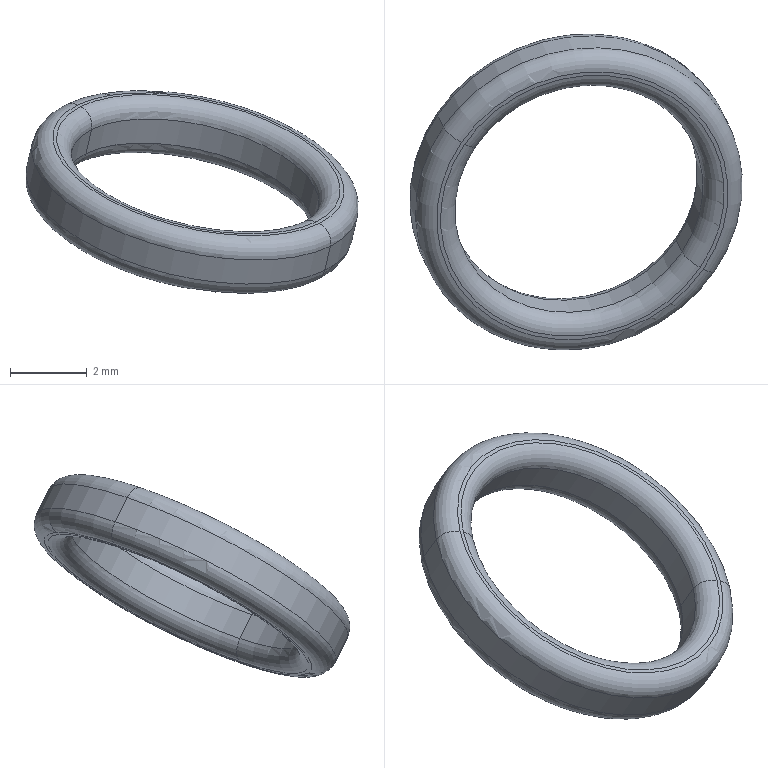Part | SolidWorks | features BaseBody 1 | 1 solid | 14 faces | box 8.65 x 8.202 x 5.272 mm | volume 36.271 mm3 | torus 8 | cylinder 4 | plane 2 | commonest cylinder face diameters 6.6 x2 8.665 x2
STEP:
#1=CARTESIAN_POINT('',(1964.802,-244.96,1000.506));
#2=VERTEX_POINT('',#1);
#3=CARTESIAN_POINT('',(1970.925,-248.162,997.508));
#4=VERTEX_POINT('',#3);
#5=CARTESIAN_POINT('',(1967.864,-246.561,999.007));
#6=DIRECTION('',(-0.2015,0.436,-0.8771));
#7=DIRECTION('',(-0.9754,-0.007201,0.2205));
#8=AXIS2_PLACEMENT_3D('',#5,#6,#7);
#9=CIRCLE('',#8,3.766);
#10=EDGE_CURVE('',#2,#4,#9,.T.);
#11=ORIENTED_EDGE('',*,*,#10,.F.);
#12=CARTESIAN_POINT('',(1965.087,-244.955,999.912));
#13=VERTEX_POINT('',#12);
#14=CARTESIAN_POINT('',(1964.708,-244.757,1000.097));
#15=DIRECTION('',(-0.5464,-0.7932,-0.2688));
#16=DIRECTION('',(-0.8129,0.4251,0.3981));
#17=AXIS2_PLACEMENT_3D('',#14,#15,#16);
#18=CIRCLE('',#17,0.4662);
#19=EDGE_CURVE('',#13,#2,#18,.T.);
#20=ORIENTED_EDGE('',*,*,#19,.F.);
#21=CARTESIAN_POINT('',(1970.452,-247.761,997.284));
#22=VERTEX_POINT('',#21);
#23=CARTESIAN_POINT('',(1967.77,-246.358,998.598));
#24=DIRECTION('',(-0.2015,0.436,-0.8771));
#25=DIRECTION('',(-0.9754,-0.007201,0.2205));
#26=AXIS2_PLACEMENT_3D('',#23,#24,#25);
#27=CIRCLE('',#26,3.3);
#28=EDGE_CURVE('',#13,#22,#27,.T.);
#29=ORIENTED_EDGE('',*,*,#28,.T.);
#30=CARTESIAN_POINT('',(1970.831,-247.959,997.099));
#31=DIRECTION('',(-0.5464,-0.7932,-0.2688));
#32=DIRECTION('',(-0.8129,0.4251,0.3981));
#33=AXIS2_PLACEMENT_3D('',#30,#31,#32);
#34=CIRCLE('',#33,0.4663);
#35=EDGE_CURVE('',#4,#22,#34,.T.);
#36=ORIENTED_EDGE('',*,*,#35,.F.);
#37=EDGE_LOOP('',(#11,#20,#29,#36));
#38=FACE_OUTER_BOUND('',#37,.T.);
#39=CARTESIAN_POINT('',(1967.77,-246.358,998.598));
#40=DIRECTION('',(-0.2015,0.436,-0.8771));
#41=DIRECTION('',(0.8129,-0.4251,-0.3981));
#42=AXIS2_PLACEMENT_3D('',#39,#40,#41);
#43=TOROIDAL_SURFACE('',#42,3.766,0.4662);
#44=ADVANCED_FACE('',(#38),#43,.T.);
#45=CARTESIAN_POINT('',(1967.864,-246.561,999.007));
#46=DIRECTION('',(-0.2015,0.436,-0.8771));
#47=DIRECTION('',(-0.9754,-0.007201,0.2205));
#48=AXIS2_PLACEMENT_3D('',#45,#46,#47);
#49=CIRCLE('',#48,3.766);
#50=EDGE_CURVE('',#4,#2,#49,.T.);
#51=ORIENTED_EDGE('',*,*,#50,.F.);
#52=ORIENTED_EDGE('',*,*,#35,.T.);
#53=CARTESIAN_POINT('',(1967.77,-246.358,998.598));
#54=DIRECTION('',(-0.2015,0.436,-0.8771));
#55=DIRECTION('',(-0.9754,-0.007201,0.2205));
#56=AXIS2_PLACEMENT_3D('',#53,#54,#55);
#57=CIRCLE('',#56,3.3);
#58=EDGE_CURVE('',#22,#13,#57,.T.);
#59=ORIENTED_EDGE('',*,*,#58,.T.);
#60=ORIENTED_EDGE('',*,*,#19,.T.);
#61=EDGE_LOOP('',(#51,#52,#59,#60));
#62=FACE_OUTER_BOUND('',#61,.T.);
#63=CARTESIAN_POINT('',(1967.77,-246.358,998.598));
#64=DIRECTION('',(-0.2015,0.436,-0.8771));
#65=DIRECTION('',(0.8129,-0.4251,-0.3981));
#66=AXIS2_PLACEMENT_3D('',#63,#64,#65);
#67=TOROIDAL_SURFACE('',#66,3.766,0.4662);
#68=ADVANCED_FACE('',(#62),#67,.T.);
#69=ORIENTED_EDGE('',*,*,#28,.F.);
#70=CARTESIAN_POINT('',(1964.943,-244.644,999.286));
#71=VERTEX_POINT('',#70);
#72=CARTESIAN_POINT('',(1965.015,-244.8,999.599));
#73=DIRECTION('',(-0.2015,0.436,-0.8771));
#74=VECTOR('',#73,1000.);
#75=LINE('',#72,#74);
#76=EDGE_CURVE('',#13,#71,#75,.T.);
#77=ORIENTED_EDGE('',*,*,#76,.T.);
#78=CARTESIAN_POINT('',(1970.309,-247.45,996.659));
#79=VERTEX_POINT('',#78);
#80=CARTESIAN_POINT('',(1967.626,-246.047,997.973));
#81=DIRECTION('',(-0.2015,0.436,-0.8771));
#82=DIRECTION('',(-0.9754,-0.007201,0.2205));
#83=AXIS2_PLACEMENT_3D('',#80,#81,#82);
#84=CIRCLE('',#83,3.3);
#85=EDGE_CURVE('',#71,#79,#84,.T.);
#86=ORIENTED_EDGE('',*,*,#85,.T.);
#87=CARTESIAN_POINT('',(1970.38,-247.605,996.972));
#88=DIRECTION('',(0.2015,-0.436,0.8771));
#89=VECTOR('',#88,1000.);
#90=LINE('',#87,#89);
#91=EDGE_CURVE('',#79,#22,#90,.T.);
#92=ORIENTED_EDGE('',*,*,#91,.T.);
#93=EDGE_LOOP('',(#69,#77,#86,#92));
#94=FACE_OUTER_BOUND('',#93,.T.);
#95=CARTESIAN_POINT('',(1967.698,-246.203,998.285));
#96=DIRECTION('',(-0.2015,0.436,-0.8771));
#97=DIRECTION('',(0.8129,-0.4251,-0.3981));
#98=AXIS2_PLACEMENT_3D('',#95,#96,#97);
#99=CYLINDRICAL_SURFACE('',#98,3.3);
#100=ADVANCED_FACE('',(#94),#99,.F.);
#101=ORIENTED_EDGE('',*,*,#58,.F.);
#102=ORIENTED_EDGE('',*,*,#91,.F.);
#103=CARTESIAN_POINT('',(1967.626,-246.047,997.973));
#104=DIRECTION('',(-0.2015,0.436,-0.8771));
#105=DIRECTION('',(-0.9754,-0.007201,0.2205));
#106=AXIS2_PLACEMENT_3D('',#103,#104,#105);
#107=CIRCLE('',#106,3.3);
#108=EDGE_CURVE('',#79,#71,#107,.T.);
#109=ORIENTED_EDGE('',*,*,#108,.T.);
#110=ORIENTED_EDGE('',*,*,#76,.F.);
#111=EDGE_LOOP('',(#101,#102,#109,#110));
#112=FACE_OUTER_BOUND('',#111,.T.);
#113=CARTESIAN_POINT('',(1967.698,-246.203,998.285));
#114=DIRECTION('',(-0.2015,0.436,-0.8771));
#115=DIRECTION('',(0.8129,-0.4251,-0.3981));
#116=AXIS2_PLACEMENT_3D('',#113,#114,#115);
#117=CYLINDRICAL_SURFACE('',#116,3.3);
#118=ADVANCED_FACE('',(#112),#117,.F.);
#119=ORIENTED_EDGE('',*,*,#85,.F.);
#120=CARTESIAN_POINT('',(1964.47,-244.243,999.063));
#121=VERTEX_POINT('',#120);
#122=CARTESIAN_POINT('',(1964.564,-244.446,999.472));
#123=DIRECTION('',(-0.5464,-0.7932,-0.2688));
#124=DIRECTION('',(-0.8129,0.4251,0.3981));
#125=AXIS2_PLACEMENT_3D('',#122,#123,#124);
#126=CIRCLE('',#125,0.4663);
#127=EDGE_CURVE('',#121,#71,#126,.T.);
#128=ORIENTED_EDGE('',*,*,#127,.F.);
#129=CARTESIAN_POINT('',(1970.594,-247.445,996.064));
#130=VERTEX_POINT('',#129);
#131=CARTESIAN_POINT('',(1967.532,-245.844,997.564));
#132=DIRECTION('',(-0.2015,0.436,-0.8771));
#133=DIRECTION('',(-0.9754,-0.007201,0.2205));
#134=AXIS2_PLACEMENT_3D('',#131,#132,#133);
#135=CIRCLE('',#134,3.766);
#136=EDGE_CURVE('',#121,#130,#135,.T.);
#137=ORIENTED_EDGE('',*,*,#136,.T.);
#138=CARTESIAN_POINT('',(1970.688,-247.648,996.473));
#139=DIRECTION('',(-0.5464,-0.7932,-0.2688));
#140=DIRECTION('',(-0.8129,0.4251,0.3981));
#141=AXIS2_PLACEMENT_3D('',#138,#139,#140);
#142=CIRCLE('',#141,0.4663);
#143=EDGE_CURVE('',#79,#130,#142,.T.);
#144=ORIENTED_EDGE('',*,*,#143,.F.);
#145=EDGE_LOOP('',(#119,#128,#137,#144));
#146=FACE_OUTER_BOUND('',#145,.T.);
#147=CARTESIAN_POINT('',(1967.626,-246.047,997.973));
#148=DIRECTION('',(-0.2015,0.436,-0.8771));
#149=DIRECTION('',(0.8129,-0.4251,-0.3981));
#150=AXIS2_PLACEMENT_3D('',#147,#148,#149);
#151=TOROIDAL_SURFACE('',#150,3.766,0.4662);
#152=ADVANCED_FACE('',(#146),#151,.T.);
#153=ORIENTED_EDGE('',*,*,#108,.F.);
#154=ORIENTED_EDGE('',*,*,#143,.T.);
#155=CARTESIAN_POINT('',(1967.532,-245.844,997.564));
#156=DIRECTION('',(-0.2015,0.436,-0.8771));
#157=DIRECTION('',(-0.9754,-0.007201,0.2205));
#158=AXIS2_PLACEMENT_3D('',#155,#156,#157);
#159=CIRCLE('',#158,3.766);
#160=EDGE_CURVE('',#130,#121,#159,.T.);
#161=ORIENTED_EDGE('',*,*,#160,.T.);
#162=ORIENTED_EDGE('',*,*,#127,.T.);
#163=EDGE_LOOP('',(#153,#154,#161,#162));
#164=FACE_OUTER_BOUND('',#163,.T.);
#165=CARTESIAN_POINT('',(1967.626,-246.047,997.973));
#166=DIRECTION('',(-0.2015,0.436,-0.8771));
#167=DIRECTION('',(0.8129,-0.4251,-0.3981));
#168=AXIS2_PLACEMENT_3D('',#165,#166,#167);
#169=TOROIDAL_SURFACE('',#168,3.766,0.4662);
#170=ADVANCED_FACE('',(#164),#169,.T.);
#171=CARTESIAN_POINT('',(1964.389,-244.2,999.103));
#172=VERTEX_POINT('',#171);
#173=CARTESIAN_POINT('',(1970.675,-247.487,996.025));
#174=VERTEX_POINT('',#173);
#175=CARTESIAN_POINT('',(1967.532,-245.844,997.564));
#176=DIRECTION('',(-0.2015,0.436,-0.8771));
#177=DIRECTION('',(-0.9754,-0.007201,0.2205));
#178=AXIS2_PLACEMENT_3D('',#175,#176,#177);
#179=CIRCLE('',#178,3.866);
#180=EDGE_CURVE('',#172,#174,#179,.T.);
#181=ORIENTED_EDGE('',*,*,#180,.F.);
#182=CARTESIAN_POINT('',(1964.104,-244.205,999.697));
#183=VERTEX_POINT('',#182);
#184=CARTESIAN_POINT('',(1964.483,-244.403,999.512));
#185=DIRECTION('',(-0.5464,-0.7932,-0.2688));
#186=DIRECTION('',(-0.8129,0.4251,0.3981));
#187=AXIS2_PLACEMENT_3D('',#184,#185,#186);
#188=CIRCLE('',#187,0.4662);
#189=EDGE_CURVE('',#183,#172,#188,.T.);
#190=ORIENTED_EDGE('',*,*,#189,.F.);
#191=CARTESIAN_POINT('',(1971.148,-247.889,996.248));
#192=VERTEX_POINT('',#191);
#193=CARTESIAN_POINT('',(1967.626,-246.047,997.973));
#194=DIRECTION('',(-0.2015,0.436,-0.8771));
#195=DIRECTION('',(-0.9754,-0.007201,0.2205));
#196=AXIS2_PLACEMENT_3D('',#193,#194,#195);
#197=CIRCLE('',#196,4.333);
#198=EDGE_CURVE('',#183,#192,#197,.T.);
#199=ORIENTED_EDGE('',*,*,#198,.T.);
#200=CARTESIAN_POINT('',(1970.769,-247.691,996.433));
#201=DIRECTION('',(-0.5464,-0.7932,-0.2688));
#202=DIRECTION('',(-0.8129,0.4251,0.3981));
#203=AXIS2_PLACEMENT_3D('',#200,#201,#202);
#204=CIRCLE('',#203,0.4663);
#205=EDGE_CURVE('',#174,#192,#204,.T.);
#206=ORIENTED_EDGE('',*,*,#205,.F.);
#207=EDGE_LOOP('',(#181,#190,#199,#206));
#208=FACE_OUTER_BOUND('',#207,.T.);
#209=CARTESIAN_POINT('',(1967.626,-246.047,997.973));
#210=DIRECTION('',(-0.2015,0.436,-0.8771));
#211=DIRECTION('',(0.8129,-0.4251,-0.3981));
#212=AXIS2_PLACEMENT_3D('',#209,#210,#211);
#213=TOROIDAL_SURFACE('',#212,3.866,0.4662);
#214=ADVANCED_FACE('',(#208),#213,.T.);
#215=CARTESIAN_POINT('',(1967.532,-245.844,997.564));
#216=DIRECTION('',(-0.2015,0.436,-0.8771));
#217=DIRECTION('',(-0.9754,-0.007201,0.2205));
#218=AXIS2_PLACEMENT_3D('',#215,#216,#217);
#219=CIRCLE('',#218,3.866);
#220=EDGE_CURVE('',#174,#172,#219,.T.);
#221=ORIENTED_EDGE('',*,*,#220,.F.);
#222=ORIENTED_EDGE('',*,*,#205,.T.);
#223=CARTESIAN_POINT('',(1967.626,-246.047,997.973));
#224=DIRECTION('',(-0.2015,0.436,-0.8771));
#225=DIRECTION('',(-0.9754,-0.007201,0.2205));
#226=AXIS2_PLACEMENT_3D('',#223,#224,#225);
#227=CIRCLE('',#226,4.333);
#228=EDGE_CURVE('',#192,#183,#227,.T.);
#229=ORIENTED_EDGE('',*,*,#228,.T.);
#230=ORIENTED_EDGE('',*,*,#189,.T.);
#231=EDGE_LOOP('',(#221,#222,#229,#230));
#232=FACE_OUTER_BOUND('',#231,.T.);
#233=CARTESIAN_POINT('',(1967.626,-246.047,997.973));
#234=DIRECTION('',(-0.2015,0.436,-0.8771));
#235=DIRECTION('',(0.8129,-0.4251,-0.3981));
#236=AXIS2_PLACEMENT_3D('',#233,#234,#235);
#237=TOROIDAL_SURFACE('',#236,3.866,0.4662);
#238=ADVANCED_FACE('',(#232),#237,.T.);
#239=ORIENTED_EDGE('',*,*,#198,.F.);
#240=CARTESIAN_POINT('',(1964.248,-244.516,1000.323));
#241=VERTEX_POINT('',#240);
#242=CARTESIAN_POINT('',(1964.176,-244.361,1000.01));
#243=DIRECTION('',(0.2015,-0.436,0.8771));
#244=VECTOR('',#243,1000.);
#245=LINE('',#242,#244);
#246=EDGE_CURVE('',#183,#241,#245,.T.);
#247=ORIENTED_EDGE('',*,*,#246,.T.);
#248=CARTESIAN_POINT('',(1971.292,-248.2,996.873));
#249=VERTEX_POINT('',#248);
#250=CARTESIAN_POINT('',(1967.77,-246.358,998.598));
#251=DIRECTION('',(-0.2015,0.436,-0.8771));
#252=DIRECTION('',(-0.9754,-0.007201,0.2205));
#253=AXIS2_PLACEMENT_3D('',#250,#251,#252);
#254=CIRCLE('',#253,4.333);
#255=EDGE_CURVE('',#241,#249,#254,.T.);
#256=ORIENTED_EDGE('',*,*,#255,.T.);
#257=CARTESIAN_POINT('',(1971.22,-248.044,996.561));
#258=DIRECTION('',(-0.2015,0.436,-0.8771));
#259=VECTOR('',#258,1000.);
#260=LINE('',#257,#259);
#261=EDGE_CURVE('',#249,#192,#260,.T.);
#262=ORIENTED_EDGE('',*,*,#261,.T.);
#263=EDGE_LOOP('',(#239,#247,#256,#262));
#264=FACE_OUTER_BOUND('',#263,.T.);
#265=CARTESIAN_POINT('',(1967.698,-246.203,998.285));
#266=DIRECTION('',(-0.2015,0.436,-0.8771));
#267=DIRECTION('',(0.8129,-0.4251,-0.3981));
#268=AXIS2_PLACEMENT_3D('',#265,#266,#267);
#269=CYLINDRICAL_SURFACE('',#268,4.333);
#270=ADVANCED_FACE('',(#264),#269,.T.);
#271=ORIENTED_EDGE('',*,*,#228,.F.);
#272=ORIENTED_EDGE('',*,*,#261,.F.);
#273=CARTESIAN_POINT('',(1967.77,-246.358,998.598));
#274=DIRECTION('',(-0.2015,0.436,-0.8771));
#275=DIRECTION('',(-0.9754,-0.007201,0.2205));
#276=AXIS2_PLACEMENT_3D('',#273,#274,#275);
#277=CIRCLE('',#276,4.333);
#278=EDGE_CURVE('',#249,#241,#277,.T.);
#279=ORIENTED_EDGE('',*,*,#278,.T.);
#280=ORIENTED_EDGE('',*,*,#246,.F.);
#281=EDGE_LOOP('',(#271,#272,#279,#280));
#282=FACE_OUTER_BOUND('',#281,.T.);
#283=CARTESIAN_POINT('',(1967.698,-246.203,998.285));
#284=DIRECTION('',(-0.2015,0.436,-0.8771));
#285=DIRECTION('',(0.8129,-0.4251,-0.3981));
#286=AXIS2_PLACEMENT_3D('',#283,#284,#285);
#287=CYLINDRICAL_SURFACE('',#286,4.333);
#288=ADVANCED_FACE('',(#282),#287,.T.);
#289=ORIENTED_EDGE('',*,*,#255,.F.);
#290=CARTESIAN_POINT('',(1964.721,-244.918,1000.546));
#291=VERTEX_POINT('',#290);
#292=CARTESIAN_POINT('',(1964.627,-244.714,1000.137));
#293=DIRECTION('',(0.5464,0.7932,0.2688));
#294=DIRECTION('',(-0.8129,0.4251,0.3981));
#295=AXIS2_PLACEMENT_3D('',#292,#293,#294);
#296=CIRCLE('',#295,0.4663);
#297=EDGE_CURVE('',#241,#291,#296,.T.);
#298=ORIENTED_EDGE('',*,*,#297,.T.);
#299=CARTESIAN_POINT('',(1971.006,-248.205,997.468));
#300=VERTEX_POINT('',#299);
#301=CARTESIAN_POINT('',(1967.864,-246.561,999.007));
#302=DIRECTION('',(-0.2015,0.436,-0.8771));
#303=DIRECTION('',(-0.9754,-0.007201,0.2205));
#304=AXIS2_PLACEMENT_3D('',#301,#302,#303);
#305=CIRCLE('',#304,3.866);
#306=EDGE_CURVE('',#291,#300,#305,.T.);
#307=ORIENTED_EDGE('',*,*,#306,.T.);
#308=CARTESIAN_POINT('',(1970.913,-248.002,997.059));
#309=DIRECTION('',(0.5464,0.7932,0.2688));
#310=DIRECTION('',(-0.8129,0.4251,0.3981));
#311=AXIS2_PLACEMENT_3D('',#308,#309,#310);
#312=CIRCLE('',#311,0.4662);
#313=EDGE_CURVE('',#300,#249,#312,.T.);
#314=ORIENTED_EDGE('',*,*,#313,.T.);
#315=EDGE_LOOP('',(#289,#298,#307,#314));
#316=FACE_OUTER_BOUND('',#315,.T.);
#317=CARTESIAN_POINT('',(1967.77,-246.358,998.598));
#318=DIRECTION('',(-0.2015,0.436,-0.8771));
#319=DIRECTION('',(0.8129,-0.4251,-0.3981));
#320=AXIS2_PLACEMENT_3D('',#317,#318,#319);
#321=TOROIDAL_SURFACE('',#320,3.866,0.4662);
#322=ADVANCED_FACE('',(#316),#321,.T.);
#323=ORIENTED_EDGE('',*,*,#278,.F.);
#324=ORIENTED_EDGE('',*,*,#313,.F.);
#325=CARTESIAN_POINT('',(1967.864,-246.561,999.007));
#326=DIRECTION('',(-0.2015,0.436,-0.8771));
#327=DIRECTION('',(-0.9754,-0.007201,0.2205));
#328=AXIS2_PLACEMENT_3D('',#325,#326,#327);
#329=CIRCLE('',#328,3.866);
#330=EDGE_CURVE('',#300,#291,#329,.T.);
#331=ORIENTED_EDGE('',*,*,#330,.T.);
#332=ORIENTED_EDGE('',*,*,#297,.F.);
#333=EDGE_LOOP('',(#323,#324,#331,#332));
#334=FACE_OUTER_BOUND('',#333,.T.);
#335=CARTESIAN_POINT('',(1967.77,-246.358,998.598));
#336=DIRECTION('',(-0.2015,0.436,-0.8771));
#337=DIRECTION('',(0.8129,-0.4251,-0.3981));
#338=AXIS2_PLACEMENT_3D('',#335,#336,#337);
#339=TOROIDAL_SURFACE('',#338,3.866,0.4662);
#340=ADVANCED_FACE('',(#334),#339,.T.);
#341=ORIENTED_EDGE('',*,*,#220,.T.);
#342=ORIENTED_EDGE('',*,*,#180,.T.);
#343=EDGE_LOOP('',(#341,#342));
#344=FACE_OUTER_BOUND('',#343,.T.);
#345=ORIENTED_EDGE('',*,*,#136,.F.);
#346=ORIENTED_EDGE('',*,*,#160,.F.);
#347=EDGE_LOOP('',(#345,#346));
#348=FACE_BOUND('',#347,.T.);
#349=CARTESIAN_POINT('',(1963.761,-245.872,998.416));
#350=DIRECTION('',(-0.2015,0.436,-0.8771));
#351=DIRECTION('',(0.9754,0.007201,-0.2205));
#352=AXIS2_PLACEMENT_3D('',#349,#350,#351);
#353=PLANE('',#352);
#354=ADVANCED_FACE('',(#344,#348),#353,.T.);
#355=ORIENTED_EDGE('',*,*,#306,.F.);
#356=ORIENTED_EDGE('',*,*,#330,.F.);
#357=EDGE_LOOP('',(#355,#356));
#358=FACE_OUTER_BOUND('',#357,.T.);
#359=ORIENTED_EDGE('',*,*,#50,.T.);
#360=ORIENTED_EDGE('',*,*,#10,.T.);
#361=EDGE_LOOP('',(#359,#360));
#362=FACE_BOUND('',#361,.T.);
#363=CARTESIAN_POINT('',(1964.19,-246.588,999.837));
#364=DIRECTION('',(-0.2015,0.436,-0.8771));
#365=DIRECTION('',(0.9754,0.007201,-0.2205));
#366=AXIS2_PLACEMENT_3D('',#363,#364,#365);
#367=PLANE('',#366);
#368=ADVANCED_FACE('',(#358,#362),#367,.F.);
#369=CLOSED_SHELL('',(#44,#68,#100,#118,#152,#170,#214,#238,#270,#288,#322,#340,#354,#368));
#370=MANIFOLD_SOLID_BREP('',#369);
#371=CARTESIAN_POINT('',(0.,0.,0.));
#372=DIRECTION('',(0.,0.,1.));
#373=DIRECTION('',(1.,0.,0.));
#374=AXIS2_PLACEMENT_3D('',#371,#372,#373);
#375=(LENGTH_UNIT()NAMED_UNIT(*)SI_UNIT(.MILLI.,.METRE.));
#376=UNCERTAINTY_MEASURE_WITH_UNIT(LENGTH_MEASURE(0.00001),#375,'','');
#377=(NAMED_UNIT(*)PLANE_ANGLE_UNIT()SI_UNIT($,.RADIAN.));
#378=(NAMED_UNIT(*)SI_UNIT($,.STERADIAN.)SOLID_ANGLE_UNIT());
#379=(GEOMETRIC_REPRESENTATION_CONTEXT(3)GLOBAL_UNCERTAINTY_ASSIGNED_CONTEXT((#376))GLOBAL_UNIT_ASSIGNED_CONTEXT((#375,#377,#378))REPRESENTATION_CONTEXT('',''));
#380=ADVANCED_BREP_SHAPE_REPRESENTATION('',(#370,#374),#379);